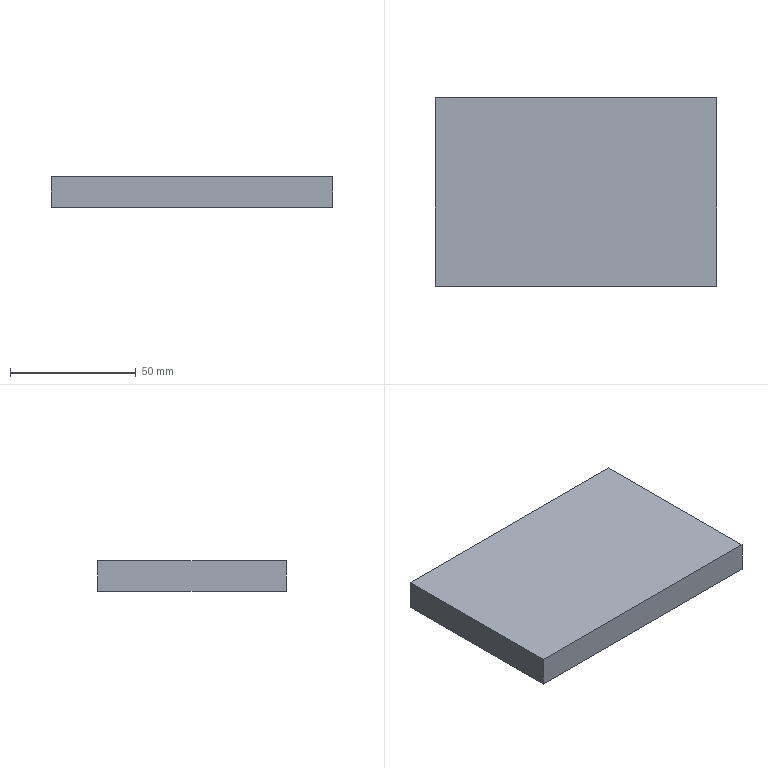Part | SolidWorks | features BaseBody 1 | 1 solid | 6 faces | box 112 x 75 x 12 mm | volume 100800 mm3 | plane 6
STEP:
#1=CARTESIAN_POINT('',(56.,-37.5,0.));
#2=VERTEX_POINT('',#1);
#3=CARTESIAN_POINT('',(56.,37.5,0.));
#4=VERTEX_POINT('',#3);
#5=CARTESIAN_POINT('',(56.,37.5,0.));
#6=DIRECTION('',(0.,1.,0.));
#7=VECTOR('',#6,1000.);
#8=LINE('',#5,#7);
#9=EDGE_CURVE('',#2,#4,#8,.T.);
#10=ORIENTED_EDGE('',*,*,#9,.T.);
#11=CARTESIAN_POINT('',(56.,37.5,12.));
#12=VERTEX_POINT('',#11);
#13=CARTESIAN_POINT('',(56.,37.5,12.));
#14=DIRECTION('',(0.,0.,-1.));
#15=VECTOR('',#14,1000.);
#16=LINE('',#13,#15);
#17=EDGE_CURVE('',#12,#4,#16,.T.);
#18=ORIENTED_EDGE('',*,*,#17,.F.);
#19=CARTESIAN_POINT('',(56.,-37.5,12.));
#20=VERTEX_POINT('',#19);
#21=CARTESIAN_POINT('',(56.,37.5,12.));
#22=DIRECTION('',(0.,1.,0.));
#23=VECTOR('',#22,1000.);
#24=LINE('',#21,#23);
#25=EDGE_CURVE('',#20,#12,#24,.T.);
#26=ORIENTED_EDGE('',*,*,#25,.F.);
#27=CARTESIAN_POINT('',(56.,-37.5,12.));
#28=DIRECTION('',(0.,0.,-1.));
#29=VECTOR('',#28,1000.);
#30=LINE('',#27,#29);
#31=EDGE_CURVE('',#20,#2,#30,.T.);
#32=ORIENTED_EDGE('',*,*,#31,.T.);
#33=EDGE_LOOP('',(#10,#18,#26,#32));
#34=FACE_OUTER_BOUND('',#33,.T.);
#35=CARTESIAN_POINT('',(56.,37.5,12.));
#36=DIRECTION('',(-1.,0.,0.));
#37=DIRECTION('',(0.,-1.,0.));
#38=AXIS2_PLACEMENT_3D('',#35,#36,#37);
#39=PLANE('',#38);
#40=ADVANCED_FACE('',(#34),#39,.F.);
#41=CARTESIAN_POINT('',(-56.,37.5,0.));
#42=VERTEX_POINT('',#41);
#43=CARTESIAN_POINT('',(-56.,37.5,0.));
#44=DIRECTION('',(-1.,0.,0.));
#45=VECTOR('',#44,1000.);
#46=LINE('',#43,#45);
#47=EDGE_CURVE('',#4,#42,#46,.T.);
#48=ORIENTED_EDGE('',*,*,#47,.T.);
#49=CARTESIAN_POINT('',(-56.,37.5,12.));
#50=VERTEX_POINT('',#49);
#51=CARTESIAN_POINT('',(-56.,37.5,12.));
#52=DIRECTION('',(0.,0.,-1.));
#53=VECTOR('',#52,1000.);
#54=LINE('',#51,#53);
#55=EDGE_CURVE('',#50,#42,#54,.T.);
#56=ORIENTED_EDGE('',*,*,#55,.F.);
#57=CARTESIAN_POINT('',(-56.,37.5,12.));
#58=DIRECTION('',(-1.,0.,0.));
#59=VECTOR('',#58,1000.);
#60=LINE('',#57,#59);
#61=EDGE_CURVE('',#12,#50,#60,.T.);
#62=ORIENTED_EDGE('',*,*,#61,.F.);
#63=ORIENTED_EDGE('',*,*,#17,.T.);
#64=EDGE_LOOP('',(#48,#56,#62,#63));
#65=FACE_OUTER_BOUND('',#64,.T.);
#66=CARTESIAN_POINT('',(-56.,37.5,12.));
#67=DIRECTION('',(0.,-1.,0.));
#68=DIRECTION('',(0.,0.,-1.));
#69=AXIS2_PLACEMENT_3D('',#66,#67,#68);
#70=PLANE('',#69);
#71=ADVANCED_FACE('',(#65),#70,.F.);
#72=CARTESIAN_POINT('',(-56.,-37.5,0.));
#73=VERTEX_POINT('',#72);
#74=CARTESIAN_POINT('',(-56.,37.5,0.));
#75=DIRECTION('',(0.,-1.,0.));
#76=VECTOR('',#75,1000.);
#77=LINE('',#74,#76);
#78=EDGE_CURVE('',#42,#73,#77,.T.);
#79=ORIENTED_EDGE('',*,*,#78,.T.);
#80=CARTESIAN_POINT('',(-56.,-37.5,12.));
#81=VERTEX_POINT('',#80);
#82=CARTESIAN_POINT('',(-56.,-37.5,12.));
#83=DIRECTION('',(0.,0.,-1.));
#84=VECTOR('',#83,1000.);
#85=LINE('',#82,#84);
#86=EDGE_CURVE('',#81,#73,#85,.T.);
#87=ORIENTED_EDGE('',*,*,#86,.F.);
#88=CARTESIAN_POINT('',(-56.,37.5,12.));
#89=DIRECTION('',(0.,-1.,0.));
#90=VECTOR('',#89,1000.);
#91=LINE('',#88,#90);
#92=EDGE_CURVE('',#50,#81,#91,.T.);
#93=ORIENTED_EDGE('',*,*,#92,.F.);
#94=ORIENTED_EDGE('',*,*,#55,.T.);
#95=EDGE_LOOP('',(#79,#87,#93,#94));
#96=FACE_OUTER_BOUND('',#95,.T.);
#97=CARTESIAN_POINT('',(-56.,37.5,12.));
#98=DIRECTION('',(1.,0.,0.));
#99=DIRECTION('',(0.,1.,0.));
#100=AXIS2_PLACEMENT_3D('',#97,#98,#99);
#101=PLANE('',#100);
#102=ADVANCED_FACE('',(#96),#101,.F.);
#103=CARTESIAN_POINT('',(-56.,-37.5,0.));
#104=DIRECTION('',(1.,0.,0.));
#105=VECTOR('',#104,1000.);
#106=LINE('',#103,#105);
#107=EDGE_CURVE('',#73,#2,#106,.T.);
#108=ORIENTED_EDGE('',*,*,#107,.T.);
#109=ORIENTED_EDGE('',*,*,#31,.F.);
#110=CARTESIAN_POINT('',(-56.,-37.5,12.));
#111=DIRECTION('',(1.,0.,0.));
#112=VECTOR('',#111,1000.);
#113=LINE('',#110,#112);
#114=EDGE_CURVE('',#81,#20,#113,.T.);
#115=ORIENTED_EDGE('',*,*,#114,.F.);
#116=ORIENTED_EDGE('',*,*,#86,.T.);
#117=EDGE_LOOP('',(#108,#109,#115,#116));
#118=FACE_OUTER_BOUND('',#117,.T.);
#119=CARTESIAN_POINT('',(-56.,-37.5,12.));
#120=DIRECTION('',(0.,1.,0.));
#121=DIRECTION('',(0.,0.,1.));
#122=AXIS2_PLACEMENT_3D('',#119,#120,#121);
#123=PLANE('',#122);
#124=ADVANCED_FACE('',(#118),#123,.F.);
#125=ORIENTED_EDGE('',*,*,#25,.T.);
#126=ORIENTED_EDGE('',*,*,#61,.T.);
#127=ORIENTED_EDGE('',*,*,#92,.T.);
#128=ORIENTED_EDGE('',*,*,#114,.T.);
#129=EDGE_LOOP('',(#125,#126,#127,#128));
#130=FACE_OUTER_BOUND('',#129,.T.);
#131=CARTESIAN_POINT('',(0.,0.,12.));
#132=DIRECTION('',(0.,0.,1.));
#133=DIRECTION('',(1.,0.,0.));
#134=AXIS2_PLACEMENT_3D('',#131,#132,#133);
#135=PLANE('',#134);
#136=ADVANCED_FACE('',(#130),#135,.T.);
#137=ORIENTED_EDGE('',*,*,#9,.F.);
#138=ORIENTED_EDGE('',*,*,#107,.F.);
#139=ORIENTED_EDGE('',*,*,#78,.F.);
#140=ORIENTED_EDGE('',*,*,#47,.F.);
#141=EDGE_LOOP('',(#137,#138,#139,#140));
#142=FACE_OUTER_BOUND('',#141,.T.);
#143=CARTESIAN_POINT('',(0.,0.,0.));
#144=DIRECTION('',(0.,0.,1.));
#145=DIRECTION('',(1.,0.,0.));
#146=AXIS2_PLACEMENT_3D('',#143,#144,#145);
#147=PLANE('',#146);
#148=ADVANCED_FACE('',(#142),#147,.F.);
#149=CLOSED_SHELL('',(#40,#71,#102,#124,#136,#148));
#150=MANIFOLD_SOLID_BREP('',#149);
#151=CARTESIAN_POINT('',(0.,0.,0.));
#152=DIRECTION('',(0.,0.,1.));
#153=DIRECTION('',(1.,0.,0.));
#154=AXIS2_PLACEMENT_3D('',#151,#152,#153);
#155=(LENGTH_UNIT()NAMED_UNIT(*)SI_UNIT(.MILLI.,.METRE.));
#156=UNCERTAINTY_MEASURE_WITH_UNIT(LENGTH_MEASURE(0.00001),#155,'','');
#157=(NAMED_UNIT(*)PLANE_ANGLE_UNIT()SI_UNIT($,.RADIAN.));
#158=(NAMED_UNIT(*)SI_UNIT($,.STERADIAN.)SOLID_ANGLE_UNIT());
#159=(GEOMETRIC_REPRESENTATION_CONTEXT(3)GLOBAL_UNCERTAINTY_ASSIGNED_CONTEXT((#156))GLOBAL_UNIT_ASSIGNED_CONTEXT((#155,#157,#158))REPRESENTATION_CONTEXT('',''));
#160=ADVANCED_BREP_SHAPE_REPRESENTATION('',(#150,#154),#159);